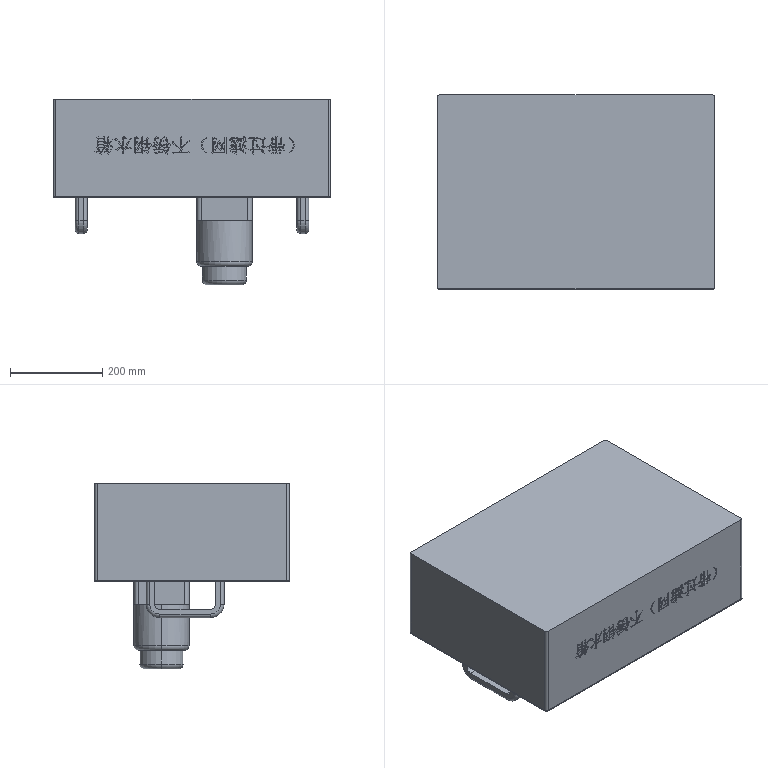Part | STEP file | PN_0002 Stainless steel water tank | 2 solids | 599 faces | box 600 x 420 x 402 mm | volume 9376328 mm3 | plane 396 | spline 155 | cylinder 36 | torus 12 | commonest cylinder face diameters 16 x12 6 x4 10 x4 20 x4 21.42 x4 58.58 x4